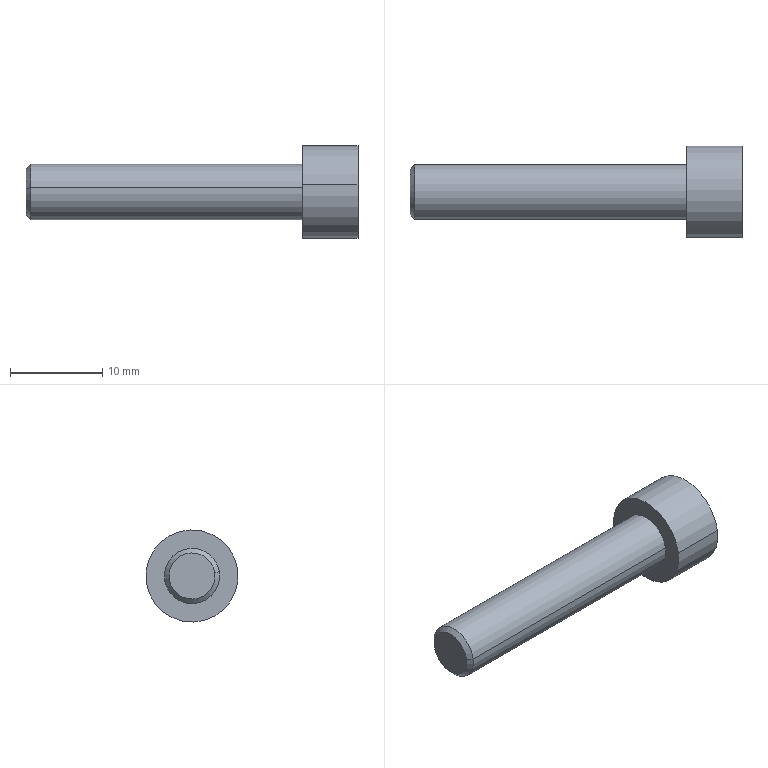Part | SolidWorks | features BaseBody 1 | 1 solid | 16 faces | box 36 x 10 x 10 mm | volume 1252 mm3 | plane 10 | cylinder 4 | cone 2 | commonest cylinder face diameters 6 x2 10 x2
STEP:
#1=CARTESIAN_POINT('',(353.4,7.47,-46.887));
#2=VERTEX_POINT('',#1);
#3=CARTESIAN_POINT('',(353.4,2.53,-46.113));
#4=VERTEX_POINT('',#3);
#5=CARTESIAN_POINT('',(353.4,5.,-46.5));
#6=DIRECTION('',(-1.,0.,0.));
#7=DIRECTION('',(0.,0.988,-0.1546));
#8=AXIS2_PLACEMENT_3D('',#5,#6,#7);
#9=CIRCLE('',#8,2.5);
#10=EDGE_CURVE('',#2,#4,#9,.T.);
#11=ORIENTED_EDGE('',*,*,#10,.F.);
#12=CARTESIAN_POINT('',(353.9,7.964,-46.964));
#13=VERTEX_POINT('',#12);
#14=CARTESIAN_POINT('',(353.4,7.47,-46.887));
#15=DIRECTION('',(0.7071,0.6986,-0.1093));
#16=VECTOR('',#15,1000.);
#17=LINE('',#14,#16);
#18=EDGE_CURVE('',#2,#13,#17,.T.);
#19=ORIENTED_EDGE('',*,*,#18,.T.);
#20=CARTESIAN_POINT('',(353.9,2.036,-46.036));
#21=VERTEX_POINT('',#20);
#22=CARTESIAN_POINT('',(353.9,5.,-46.5));
#23=DIRECTION('',(1.,0.,0.));
#24=DIRECTION('',(0.,0.988,-0.1546));
#25=AXIS2_PLACEMENT_3D('',#22,#23,#24);
#26=CIRCLE('',#25,3.);
#27=EDGE_CURVE('',#21,#13,#26,.T.);
#28=ORIENTED_EDGE('',*,*,#27,.F.);
#29=CARTESIAN_POINT('',(353.4,2.53,-46.113));
#30=DIRECTION('',(0.7071,-0.6986,0.1093));
#31=VECTOR('',#30,1000.);
#32=LINE('',#29,#31);
#33=EDGE_CURVE('',#4,#21,#32,.T.);
#34=ORIENTED_EDGE('',*,*,#33,.F.);
#35=EDGE_LOOP('',(#11,#19,#28,#34));
#36=FACE_OUTER_BOUND('',#35,.T.);
#37=CARTESIAN_POINT('',(353.4,5.,-46.5));
#38=DIRECTION('',(1.,0.,0.));
#39=DIRECTION('',(0.,-0.988,0.1546));
#40=AXIS2_PLACEMENT_3D('',#37,#38,#39);
#41=CONICAL_SURFACE('',#40,2.5,0.7854);
#42=ADVANCED_FACE('',(#36),#41,.T.);
#43=ORIENTED_EDGE('',*,*,#27,.T.);
#44=CARTESIAN_POINT('',(383.4,7.964,-46.964));
#45=VERTEX_POINT('',#44);
#46=CARTESIAN_POINT('',(353.4,7.964,-46.964));
#47=DIRECTION('',(1.,0.,0.));
#48=VECTOR('',#47,1000.);
#49=LINE('',#46,#48);
#50=EDGE_CURVE('',#13,#45,#49,.T.);
#51=ORIENTED_EDGE('',*,*,#50,.T.);
#52=CARTESIAN_POINT('',(383.4,2.036,-46.036));
#53=VERTEX_POINT('',#52);
#54=CARTESIAN_POINT('',(383.4,5.,-46.5));
#55=DIRECTION('',(-1.,0.,0.));
#56=DIRECTION('',(0.,0.988,-0.1546));
#57=AXIS2_PLACEMENT_3D('',#54,#55,#56);
#58=CIRCLE('',#57,3.);
#59=EDGE_CURVE('',#45,#53,#58,.T.);
#60=ORIENTED_EDGE('',*,*,#59,.T.);
#61=CARTESIAN_POINT('',(353.4,2.036,-46.036));
#62=DIRECTION('',(1.,0.,0.));
#63=VECTOR('',#62,1000.);
#64=LINE('',#61,#63);
#65=EDGE_CURVE('',#21,#53,#64,.T.);
#66=ORIENTED_EDGE('',*,*,#65,.F.);
#67=EDGE_LOOP('',(#43,#51,#60,#66));
#68=FACE_OUTER_BOUND('',#67,.T.);
#69=CARTESIAN_POINT('',(353.4,5.,-46.5));
#70=DIRECTION('',(1.,0.,0.));
#71=DIRECTION('',(0.,-0.988,0.1546));
#72=AXIS2_PLACEMENT_3D('',#69,#70,#71);
#73=CYLINDRICAL_SURFACE('',#72,3.);
#74=ADVANCED_FACE('',(#68),#73,.T.);
#75=CARTESIAN_POINT('',(383.4,9.94,-47.273));
#76=VERTEX_POINT('',#75);
#77=CARTESIAN_POINT('',(383.4,0.06014,-45.727));
#78=VERTEX_POINT('',#77);
#79=CARTESIAN_POINT('',(383.4,5.,-46.5));
#80=DIRECTION('',(-1.,0.,0.));
#81=DIRECTION('',(0.,0.988,-0.1546));
#82=AXIS2_PLACEMENT_3D('',#79,#80,#81);
#83=CIRCLE('',#82,5.);
#84=EDGE_CURVE('',#76,#78,#83,.T.);
#85=ORIENTED_EDGE('',*,*,#84,.F.);
#86=CARTESIAN_POINT('',(389.4,9.94,-47.273));
#87=VERTEX_POINT('',#86);
#88=CARTESIAN_POINT('',(383.4,9.94,-47.273));
#89=DIRECTION('',(1.,0.,0.));
#90=VECTOR('',#89,1000.);
#91=LINE('',#88,#90);
#92=EDGE_CURVE('',#76,#87,#91,.T.);
#93=ORIENTED_EDGE('',*,*,#92,.T.);
#94=CARTESIAN_POINT('',(389.4,0.06014,-45.727));
#95=VERTEX_POINT('',#94);
#96=CARTESIAN_POINT('',(389.4,5.,-46.5));
#97=DIRECTION('',(-1.,0.,0.));
#98=DIRECTION('',(0.,0.988,-0.1546));
#99=AXIS2_PLACEMENT_3D('',#96,#97,#98);
#100=CIRCLE('',#99,5.);
#101=EDGE_CURVE('',#87,#95,#100,.T.);
#102=ORIENTED_EDGE('',*,*,#101,.T.);
#103=CARTESIAN_POINT('',(383.4,0.06014,-45.727));
#104=DIRECTION('',(1.,0.,0.));
#105=VECTOR('',#104,1000.);
#106=LINE('',#103,#105);
#107=EDGE_CURVE('',#78,#95,#106,.T.);
#108=ORIENTED_EDGE('',*,*,#107,.F.);
#109=EDGE_LOOP('',(#85,#93,#102,#108));
#110=FACE_OUTER_BOUND('',#109,.T.);
#111=CARTESIAN_POINT('',(383.4,5.,-46.5));
#112=DIRECTION('',(1.,0.,0.));
#113=DIRECTION('',(0.,-0.988,0.1546));
#114=AXIS2_PLACEMENT_3D('',#111,#112,#113);
#115=CYLINDRICAL_SURFACE('',#114,5.);
#116=ADVANCED_FACE('',(#110),#115,.T.);
#117=CARTESIAN_POINT('',(383.4,5.,-46.5));
#118=DIRECTION('',(-1.,0.,0.));
#119=DIRECTION('',(0.,0.988,-0.1546));
#120=AXIS2_PLACEMENT_3D('',#117,#118,#119);
#121=CIRCLE('',#120,5.);
#122=EDGE_CURVE('',#78,#76,#121,.T.);
#123=ORIENTED_EDGE('',*,*,#122,.T.);
#124=ORIENTED_EDGE('',*,*,#84,.T.);
#125=EDGE_LOOP('',(#123,#124));
#126=FACE_OUTER_BOUND('',#125,.T.);
#127=CARTESIAN_POINT('',(383.4,5.,-46.5));
#128=DIRECTION('',(-1.,0.,0.));
#129=DIRECTION('',(0.,0.988,-0.1546));
#130=AXIS2_PLACEMENT_3D('',#127,#128,#129);
#131=CIRCLE('',#130,3.);
#132=EDGE_CURVE('',#53,#45,#131,.T.);
#133=ORIENTED_EDGE('',*,*,#132,.F.);
#134=ORIENTED_EDGE('',*,*,#59,.F.);
#135=EDGE_LOOP('',(#133,#134));
#136=FACE_BOUND('',#135,.T.);
#137=CARTESIAN_POINT('',(383.4,5.,-46.5));
#138=DIRECTION('',(-1.,0.,0.));
#139=DIRECTION('',(0.,0.988,-0.1546));
#140=AXIS2_PLACEMENT_3D('',#137,#138,#139);
#141=PLANE('',#140);
#142=ADVANCED_FACE('',(#126,#136),#141,.T.);
#143=ORIENTED_EDGE('',*,*,#92,.F.);
#144=ORIENTED_EDGE('',*,*,#122,.F.);
#145=ORIENTED_EDGE('',*,*,#107,.T.);
#146=CARTESIAN_POINT('',(389.4,5.,-46.5));
#147=DIRECTION('',(-1.,0.,0.));
#148=DIRECTION('',(0.,0.988,-0.1546));
#149=AXIS2_PLACEMENT_3D('',#146,#147,#148);
#150=CIRCLE('',#149,5.);
#151=EDGE_CURVE('',#95,#87,#150,.T.);
#152=ORIENTED_EDGE('',*,*,#151,.T.);
#153=EDGE_LOOP('',(#143,#144,#145,#152));
#154=FACE_OUTER_BOUND('',#153,.T.);
#155=CARTESIAN_POINT('',(383.4,5.,-46.5));
#156=DIRECTION('',(1.,0.,0.));
#157=DIRECTION('',(0.,-0.988,0.1546));
#158=AXIS2_PLACEMENT_3D('',#155,#156,#157);
#159=CYLINDRICAL_SURFACE('',#158,5.);
#160=ADVANCED_FACE('',(#154),#159,.T.);
#161=CARTESIAN_POINT('',(389.4,7.247,-48.313));
#162=VERTEX_POINT('',#161);
#163=CARTESIAN_POINT('',(389.4,7.693,-45.461));
#164=VERTEX_POINT('',#163);
#165=CARTESIAN_POINT('',(389.4,7.247,-48.313));
#166=DIRECTION('',(0.,0.1546,0.988));
#167=VECTOR('',#166,1000.);
#168=LINE('',#165,#167);
#169=EDGE_CURVE('',#162,#164,#168,.T.);
#170=ORIENTED_EDGE('',*,*,#169,.F.);
#171=CARTESIAN_POINT('',(389.4,4.554,-49.352));
#172=VERTEX_POINT('',#171);
#173=CARTESIAN_POINT('',(389.4,4.554,-49.352));
#174=DIRECTION('',(0.,0.9329,0.3601));
#175=VECTOR('',#174,1000.);
#176=LINE('',#173,#175);
#177=EDGE_CURVE('',#172,#162,#176,.T.);
#178=ORIENTED_EDGE('',*,*,#177,.F.);
#179=CARTESIAN_POINT('',(389.4,2.307,-47.539));
#180=VERTEX_POINT('',#179);
#181=CARTESIAN_POINT('',(389.4,4.554,-49.352));
#182=DIRECTION('',(0.,0.7783,-0.6279));
#183=VECTOR('',#182,1000.);
#184=LINE('',#181,#183);
#185=EDGE_CURVE('',#180,#172,#184,.T.);
#186=ORIENTED_EDGE('',*,*,#185,.F.);
#187=CARTESIAN_POINT('',(389.4,2.753,-44.687));
#188=VERTEX_POINT('',#187);
#189=CARTESIAN_POINT('',(389.4,2.307,-47.539));
#190=DIRECTION('',(0.,-0.1546,-0.988));
#191=VECTOR('',#190,1000.);
#192=LINE('',#189,#191);
#193=EDGE_CURVE('',#188,#180,#192,.T.);
#194=ORIENTED_EDGE('',*,*,#193,.F.);
#195=CARTESIAN_POINT('',(389.4,5.446,-43.648));
#196=VERTEX_POINT('',#195);
#197=CARTESIAN_POINT('',(389.4,5.446,-43.648));
#198=DIRECTION('',(0.,-0.9329,-0.3601));
#199=VECTOR('',#198,1000.);
#200=LINE('',#197,#199);
#201=EDGE_CURVE('',#196,#188,#200,.T.);
#202=ORIENTED_EDGE('',*,*,#201,.F.);
#203=CARTESIAN_POINT('',(389.4,5.446,-43.648));
#204=DIRECTION('',(0.,-0.7783,0.6279));
#205=VECTOR('',#204,1000.);
#206=LINE('',#203,#205);
#207=EDGE_CURVE('',#164,#196,#206,.T.);
#208=ORIENTED_EDGE('',*,*,#207,.F.);
#209=EDGE_LOOP('',(#170,#178,#186,#194,#202,#208));
#210=FACE_BOUND('',#209,.T.);
#211=ORIENTED_EDGE('',*,*,#151,.F.);
#212=ORIENTED_EDGE('',*,*,#101,.F.);
#213=EDGE_LOOP('',(#211,#212));
#214=FACE_OUTER_BOUND('',#213,.T.);
#215=CARTESIAN_POINT('',(389.4,5.,-46.5));
#216=DIRECTION('',(-1.,0.,0.));
#217=DIRECTION('',(0.,0.988,-0.1546));
#218=AXIS2_PLACEMENT_3D('',#215,#216,#217);
#219=PLANE('',#218);
#220=ADVANCED_FACE('',(#210,#214),#219,.F.);
#221=ORIENTED_EDGE('',*,*,#50,.F.);
#222=CARTESIAN_POINT('',(353.9,5.,-46.5));
#223=DIRECTION('',(1.,0.,0.));
#224=DIRECTION('',(0.,0.988,-0.1546));
#225=AXIS2_PLACEMENT_3D('',#222,#223,#224);
#226=CIRCLE('',#225,3.);
#227=EDGE_CURVE('',#13,#21,#226,.T.);
#228=ORIENTED_EDGE('',*,*,#227,.T.);
#229=ORIENTED_EDGE('',*,*,#65,.T.);
#230=ORIENTED_EDGE('',*,*,#132,.T.);
#231=EDGE_LOOP('',(#221,#228,#229,#230));
#232=FACE_OUTER_BOUND('',#231,.T.);
#233=CARTESIAN_POINT('',(353.4,5.,-46.5));
#234=DIRECTION('',(1.,0.,0.));
#235=DIRECTION('',(0.,-0.988,0.1546));
#236=AXIS2_PLACEMENT_3D('',#233,#234,#235);
#237=CYLINDRICAL_SURFACE('',#236,3.);
#238=ADVANCED_FACE('',(#232),#237,.T.);
#239=CARTESIAN_POINT('',(353.4,5.,-46.5));
#240=DIRECTION('',(-1.,0.,0.));
#241=DIRECTION('',(0.,0.988,-0.1546));
#242=AXIS2_PLACEMENT_3D('',#239,#240,#241);
#243=CIRCLE('',#242,2.5);
#244=EDGE_CURVE('',#4,#2,#243,.T.);
#245=ORIENTED_EDGE('',*,*,#244,.T.);
#246=ORIENTED_EDGE('',*,*,#10,.T.);
#247=EDGE_LOOP('',(#245,#246));
#248=FACE_OUTER_BOUND('',#247,.T.);
#249=CARTESIAN_POINT('',(353.4,5.,-46.5));
#250=DIRECTION('',(-1.,0.,0.));
#251=DIRECTION('',(0.,0.988,-0.1546));
#252=AXIS2_PLACEMENT_3D('',#249,#250,#251);
#253=PLANE('',#252);
#254=ADVANCED_FACE('',(#248),#253,.T.);
#255=ORIENTED_EDGE('',*,*,#177,.T.);
#256=CARTESIAN_POINT('',(386.4,7.247,-48.313));
#257=VERTEX_POINT('',#256);
#258=CARTESIAN_POINT('',(386.4,7.247,-48.313));
#259=DIRECTION('',(1.,0.,0.));
#260=VECTOR('',#259,1000.);
#261=LINE('',#258,#260);
#262=EDGE_CURVE('',#257,#162,#261,.T.);
#263=ORIENTED_EDGE('',*,*,#262,.F.);
#264=CARTESIAN_POINT('',(386.4,4.554,-49.352));
#265=VERTEX_POINT('',#264);
#266=CARTESIAN_POINT('',(386.4,4.554,-49.352));
#267=DIRECTION('',(0.,0.9329,0.3601));
#268=VECTOR('',#267,1000.);
#269=LINE('',#266,#268);
#270=EDGE_CURVE('',#265,#257,#269,.T.);
#271=ORIENTED_EDGE('',*,*,#270,.F.);
#272=CARTESIAN_POINT('',(386.4,4.554,-49.352));
#273=DIRECTION('',(1.,0.,0.));
#274=VECTOR('',#273,1000.);
#275=LINE('',#272,#274);
#276=EDGE_CURVE('',#265,#172,#275,.T.);
#277=ORIENTED_EDGE('',*,*,#276,.T.);
#278=EDGE_LOOP('',(#255,#263,#271,#277));
#279=FACE_OUTER_BOUND('',#278,.T.);
#280=CARTESIAN_POINT('',(386.4,4.554,-49.352));
#281=DIRECTION('',(0.,0.3601,-0.9329));
#282=DIRECTION('',(0.,-0.9329,-0.3601));
#283=AXIS2_PLACEMENT_3D('',#280,#281,#282);
#284=PLANE('',#283);
#285=ADVANCED_FACE('',(#279),#284,.F.);
#286=ORIENTED_EDGE('',*,*,#185,.T.);
#287=ORIENTED_EDGE('',*,*,#276,.F.);
#288=CARTESIAN_POINT('',(386.4,2.307,-47.539));
#289=VERTEX_POINT('',#288);
#290=CARTESIAN_POINT('',(386.4,4.554,-49.352));
#291=DIRECTION('',(0.,0.7783,-0.6279));
#292=VECTOR('',#291,1000.);
#293=LINE('',#290,#292);
#294=EDGE_CURVE('',#289,#265,#293,.T.);
#295=ORIENTED_EDGE('',*,*,#294,.F.);
#296=CARTESIAN_POINT('',(386.4,2.307,-47.539));
#297=DIRECTION('',(1.,0.,0.));
#298=VECTOR('',#297,1000.);
#299=LINE('',#296,#298);
#300=EDGE_CURVE('',#289,#180,#299,.T.);
#301=ORIENTED_EDGE('',*,*,#300,.T.);
#302=EDGE_LOOP('',(#286,#287,#295,#301));
#303=FACE_OUTER_BOUND('',#302,.T.);
#304=CARTESIAN_POINT('',(386.4,4.554,-49.352));
#305=DIRECTION('',(0.,-0.6279,-0.7783));
#306=DIRECTION('',(0.,-0.7783,0.6279));
#307=AXIS2_PLACEMENT_3D('',#304,#305,#306);
#308=PLANE('',#307);
#309=ADVANCED_FACE('',(#303),#308,.F.);
#310=ORIENTED_EDGE('',*,*,#193,.T.);
#311=ORIENTED_EDGE('',*,*,#300,.F.);
#312=CARTESIAN_POINT('',(386.4,2.753,-44.687));
#313=VERTEX_POINT('',#312);
#314=CARTESIAN_POINT('',(386.4,2.307,-47.539));
#315=DIRECTION('',(0.,-0.1546,-0.988));
#316=VECTOR('',#315,1000.);
#317=LINE('',#314,#316);
#318=EDGE_CURVE('',#313,#289,#317,.T.);
#319=ORIENTED_EDGE('',*,*,#318,.F.);
#320=CARTESIAN_POINT('',(386.4,2.753,-44.687));
#321=DIRECTION('',(1.,0.,0.));
#322=VECTOR('',#321,1000.);
#323=LINE('',#320,#322);
#324=EDGE_CURVE('',#313,#188,#323,.T.);
#325=ORIENTED_EDGE('',*,*,#324,.T.);
#326=EDGE_LOOP('',(#310,#311,#319,#325));
#327=FACE_OUTER_BOUND('',#326,.T.);
#328=CARTESIAN_POINT('',(386.4,2.307,-47.539));
#329=DIRECTION('',(0.,-0.988,0.1546));
#330=DIRECTION('',(-1.,0.,0.));
#331=AXIS2_PLACEMENT_3D('',#328,#329,#330);
#332=PLANE('',#331);
#333=ADVANCED_FACE('',(#327),#332,.F.);
#334=ORIENTED_EDGE('',*,*,#201,.T.);
#335=ORIENTED_EDGE('',*,*,#324,.F.);
#336=CARTESIAN_POINT('',(386.4,5.446,-43.648));
#337=VERTEX_POINT('',#336);
#338=CARTESIAN_POINT('',(386.4,5.446,-43.648));
#339=DIRECTION('',(0.,-0.9329,-0.3601));
#340=VECTOR('',#339,1000.);
#341=LINE('',#338,#340);
#342=EDGE_CURVE('',#337,#313,#341,.T.);
#343=ORIENTED_EDGE('',*,*,#342,.F.);
#344=CARTESIAN_POINT('',(386.4,5.446,-43.648));
#345=DIRECTION('',(1.,0.,0.));
#346=VECTOR('',#345,1000.);
#347=LINE('',#344,#346);
#348=EDGE_CURVE('',#337,#196,#347,.T.);
#349=ORIENTED_EDGE('',*,*,#348,.T.);
#350=EDGE_LOOP('',(#334,#335,#343,#349));
#351=FACE_OUTER_BOUND('',#350,.T.);
#352=CARTESIAN_POINT('',(386.4,5.446,-43.648));
#353=DIRECTION('',(0.,-0.3601,0.9329));
#354=DIRECTION('',(0.,0.9329,0.3601));
#355=AXIS2_PLACEMENT_3D('',#352,#353,#354);
#356=PLANE('',#355);
#357=ADVANCED_FACE('',(#351),#356,.F.);
#358=ORIENTED_EDGE('',*,*,#207,.T.);
#359=ORIENTED_EDGE('',*,*,#348,.F.);
#360=CARTESIAN_POINT('',(386.4,7.693,-45.461));
#361=VERTEX_POINT('',#360);
#362=CARTESIAN_POINT('',(386.4,5.446,-43.648));
#363=DIRECTION('',(0.,-0.7783,0.6279));
#364=VECTOR('',#363,1000.);
#365=LINE('',#362,#364);
#366=EDGE_CURVE('',#361,#337,#365,.T.);
#367=ORIENTED_EDGE('',*,*,#366,.F.);
#368=CARTESIAN_POINT('',(386.4,7.693,-45.461));
#369=DIRECTION('',(1.,0.,0.));
#370=VECTOR('',#369,1000.);
#371=LINE('',#368,#370);
#372=EDGE_CURVE('',#361,#164,#371,.T.);
#373=ORIENTED_EDGE('',*,*,#372,.T.);
#374=EDGE_LOOP('',(#358,#359,#367,#373));
#375=FACE_OUTER_BOUND('',#374,.T.);
#376=CARTESIAN_POINT('',(386.4,5.446,-43.648));
#377=DIRECTION('',(0.,0.6279,0.7783));
#378=DIRECTION('',(0.,0.7783,-0.6279));
#379=AXIS2_PLACEMENT_3D('',#376,#377,#378);
#380=PLANE('',#379);
#381=ADVANCED_FACE('',(#375),#380,.F.);
#382=ORIENTED_EDGE('',*,*,#169,.T.);
#383=ORIENTED_EDGE('',*,*,#372,.F.);
#384=CARTESIAN_POINT('',(386.4,7.247,-48.313));
#385=DIRECTION('',(0.,0.1546,0.988));
#386=VECTOR('',#385,1000.);
#387=LINE('',#384,#386);
#388=EDGE_CURVE('',#257,#361,#387,.T.);
#389=ORIENTED_EDGE('',*,*,#388,.F.);
#390=ORIENTED_EDGE('',*,*,#262,.T.);
#391=EDGE_LOOP('',(#382,#383,#389,#390));
#392=FACE_OUTER_BOUND('',#391,.T.);
#393=CARTESIAN_POINT('',(386.4,7.247,-48.313));
#394=DIRECTION('',(0.,0.988,-0.1546));
#395=DIRECTION('',(1.,0.,0.));
#396=AXIS2_PLACEMENT_3D('',#393,#394,#395);
#397=PLANE('',#396);
#398=ADVANCED_FACE('',(#392),#397,.F.);
#399=ORIENTED_EDGE('',*,*,#270,.T.);
#400=ORIENTED_EDGE('',*,*,#388,.T.);
#401=ORIENTED_EDGE('',*,*,#366,.T.);
#402=ORIENTED_EDGE('',*,*,#342,.T.);
#403=ORIENTED_EDGE('',*,*,#318,.T.);
#404=ORIENTED_EDGE('',*,*,#294,.T.);
#405=EDGE_LOOP('',(#399,#400,#401,#402,#403,#404));
#406=FACE_OUTER_BOUND('',#405,.T.);
#407=CARTESIAN_POINT('',(386.4,4.554,-49.352));
#408=DIRECTION('',(1.,0.,0.));
#409=DIRECTION('',(0.,-0.988,0.1546));
#410=AXIS2_PLACEMENT_3D('',#407,#408,#409);
#411=PLANE('',#410);
#412=ADVANCED_FACE('',(#406),#411,.T.);
#413=ORIENTED_EDGE('',*,*,#18,.F.);
#414=ORIENTED_EDGE('',*,*,#244,.F.);
#415=ORIENTED_EDGE('',*,*,#33,.T.);
#416=ORIENTED_EDGE('',*,*,#227,.F.);
#417=EDGE_LOOP('',(#413,#414,#415,#416));
#418=FACE_OUTER_BOUND('',#417,.T.);
#419=CARTESIAN_POINT('',(353.4,5.,-46.5));
#420=DIRECTION('',(1.,0.,0.));
#421=DIRECTION('',(0.,-0.988,0.1546));
#422=AXIS2_PLACEMENT_3D('',#419,#420,#421);
#423=CONICAL_SURFACE('',#422,2.5,0.7854);
#424=ADVANCED_FACE('',(#418),#423,.T.);
#425=CLOSED_SHELL('',(#42,#74,#116,#142,#160,#220,#238,#254,#285,#309,#333,#357,#381,#398,#412,#424));
#426=MANIFOLD_SOLID_BREP('',#425);
#427=CARTESIAN_POINT('',(0.,0.,0.));
#428=DIRECTION('',(0.,0.,1.));
#429=DIRECTION('',(1.,0.,0.));
#430=AXIS2_PLACEMENT_3D('',#427,#428,#429);
#431=(LENGTH_UNIT()NAMED_UNIT(*)SI_UNIT(.MILLI.,.METRE.));
#432=UNCERTAINTY_MEASURE_WITH_UNIT(LENGTH_MEASURE(0.00001),#431,'','');
#433=(NAMED_UNIT(*)PLANE_ANGLE_UNIT()SI_UNIT($,.RADIAN.));
#434=(NAMED_UNIT(*)SI_UNIT($,.STERADIAN.)SOLID_ANGLE_UNIT());
#435=(GEOMETRIC_REPRESENTATION_CONTEXT(3)GLOBAL_UNCERTAINTY_ASSIGNED_CONTEXT((#432))GLOBAL_UNIT_ASSIGNED_CONTEXT((#431,#433,#434))REPRESENTATION_CONTEXT('',''));
#436=ADVANCED_BREP_SHAPE_REPRESENTATION('',(#426,#430),#435);